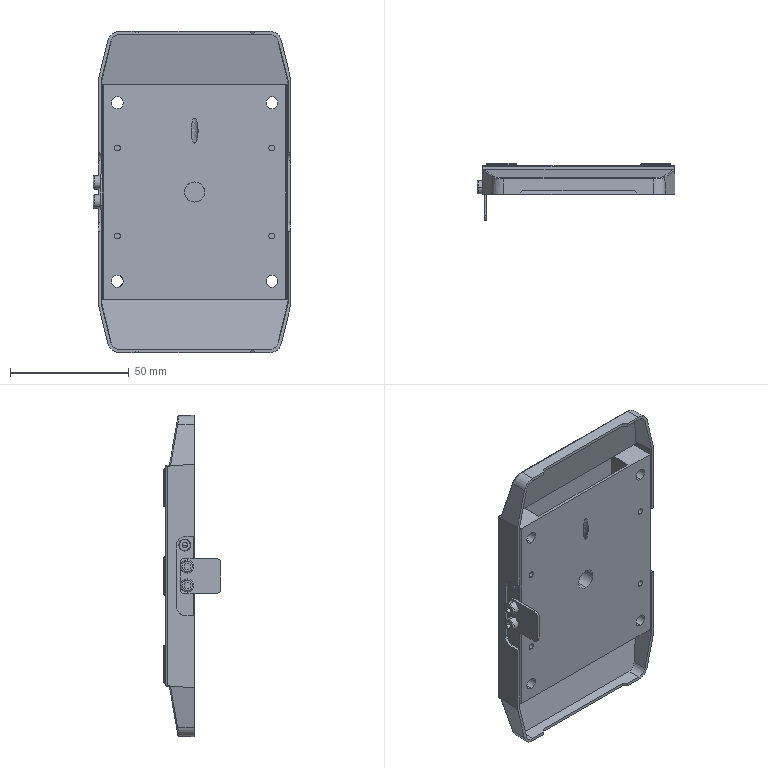Part | SolidWorks | 5 solids | 347 faces | box 83.2 x 24 x 135 mm | volume 27538 mm3 | plane 153 | cylinder 132 | spline 42 | cone 20 | commonest cylinder face diameters 1 x58 2.5 x16 5 x16 3.4 x8 5.54 x8 3.3 x4